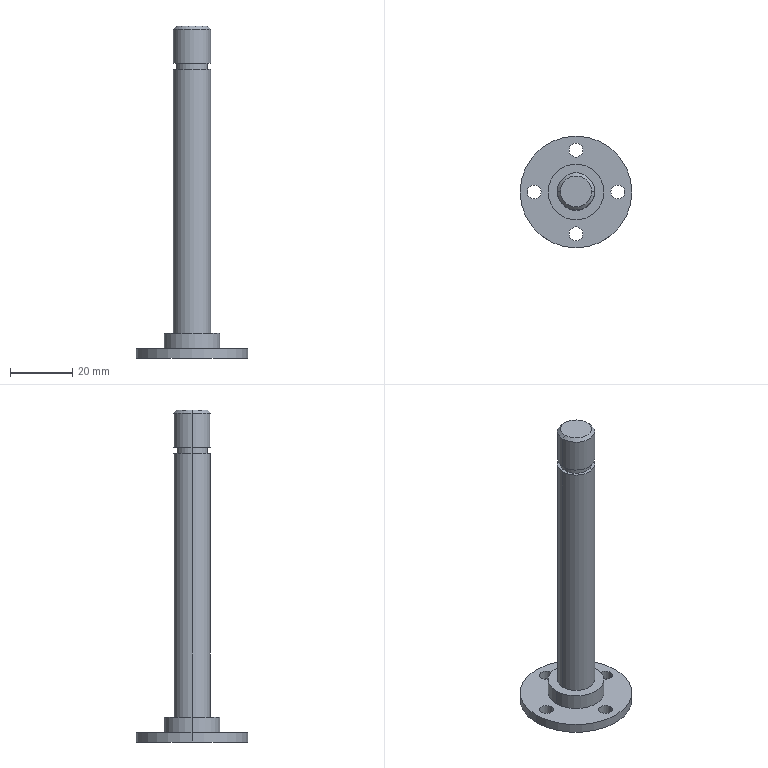Part | STEP file | Floating guide shaft | 1 solid | 26 faces | box 36 x 36 x 107 mm | volume 15245 mm3 | cylinder 18 | plane 6 | cone 2 | commonest cylinder face diameters 4.5 x8 12 x4 10 x2 18 x2 36 x2
STEP:
#1=CARTESIAN_POINT('',(5.,0.,107.));
#2=VERTEX_POINT('',#1);
#3=CARTESIAN_POINT('',(-5.,0.,107.));
#4=VERTEX_POINT('',#3);
#5=CARTESIAN_POINT('',(0.,0.,107.));
#6=DIRECTION('',(0.,0.,1.));
#7=DIRECTION('',(1.,0.,0.));
#8=AXIS2_PLACEMENT_3D('',#5,#6,#7);
#9=CIRCLE('',#8,5.);
#10=EDGE_CURVE('',#2,#4,#9,.T.);
#11=ORIENTED_EDGE('',*,*,#10,.F.);
#12=CARTESIAN_POINT('',(6.,0.,106.));
#13=VERTEX_POINT('',#12);
#14=CARTESIAN_POINT('',(5.,0.,107.));
#15=DIRECTION('',(0.7071,0.,-0.7071));
#16=VECTOR('',#15,1000.);
#17=LINE('',#14,#16);
#18=EDGE_CURVE('',#2,#13,#17,.T.);
#19=ORIENTED_EDGE('',*,*,#18,.T.);
#20=CARTESIAN_POINT('',(-6.,0.,106.));
#21=VERTEX_POINT('',#20);
#22=CARTESIAN_POINT('',(0.,0.,106.));
#23=DIRECTION('',(0.,0.,-1.));
#24=DIRECTION('',(1.,0.,0.));
#25=AXIS2_PLACEMENT_3D('',#22,#23,#24);
#26=CIRCLE('',#25,6.);
#27=EDGE_CURVE('',#21,#13,#26,.T.);
#28=ORIENTED_EDGE('',*,*,#27,.F.);
#29=CARTESIAN_POINT('',(-5.,0.,107.));
#30=DIRECTION('',(-0.7071,0.,-0.7071));
#31=VECTOR('',#30,1000.);
#32=LINE('',#29,#31);
#33=EDGE_CURVE('',#4,#21,#32,.T.);
#34=ORIENTED_EDGE('',*,*,#33,.F.);
#35=EDGE_LOOP('',(#11,#19,#28,#34));
#36=FACE_OUTER_BOUND('',#35,.T.);
#37=CARTESIAN_POINT('',(0.,0.,107.));
#38=DIRECTION('',(0.,0.,-1.));
#39=DIRECTION('',(-1.,0.,0.));
#40=AXIS2_PLACEMENT_3D('',#37,#38,#39);
#41=CONICAL_SURFACE('',#40,5.,0.7854);
#42=ADVANCED_FACE('',(#36),#41,.T.);
#43=ORIENTED_EDGE('',*,*,#27,.T.);
#44=CARTESIAN_POINT('',(6.,0.,95.));
#45=VERTEX_POINT('',#44);
#46=CARTESIAN_POINT('',(6.,0.,107.));
#47=DIRECTION('',(0.,0.,-1.));
#48=VECTOR('',#47,1000.);
#49=LINE('',#46,#48);
#50=EDGE_CURVE('',#13,#45,#49,.T.);
#51=ORIENTED_EDGE('',*,*,#50,.T.);
#52=CARTESIAN_POINT('',(-6.,0.,95.));
#53=VERTEX_POINT('',#52);
#54=CARTESIAN_POINT('',(0.,0.,95.));
#55=DIRECTION('',(0.,0.,1.));
#56=DIRECTION('',(1.,0.,0.));
#57=AXIS2_PLACEMENT_3D('',#54,#55,#56);
#58=CIRCLE('',#57,6.);
#59=EDGE_CURVE('',#45,#53,#58,.T.);
#60=ORIENTED_EDGE('',*,*,#59,.T.);
#61=CARTESIAN_POINT('',(-6.,0.,107.));
#62=DIRECTION('',(0.,0.,-1.));
#63=VECTOR('',#62,1000.);
#64=LINE('',#61,#63);
#65=EDGE_CURVE('',#21,#53,#64,.T.);
#66=ORIENTED_EDGE('',*,*,#65,.F.);
#67=EDGE_LOOP('',(#43,#51,#60,#66));
#68=FACE_OUTER_BOUND('',#67,.T.);
#69=CARTESIAN_POINT('',(0.,0.,107.));
#70=DIRECTION('',(0.,0.,-1.));
#71=DIRECTION('',(-1.,0.,0.));
#72=AXIS2_PLACEMENT_3D('',#69,#70,#71);
#73=CYLINDRICAL_SURFACE('',#72,6.);
#74=ADVANCED_FACE('',(#68),#73,.T.);
#75=CARTESIAN_POINT('',(5.,0.,95.));
#76=VERTEX_POINT('',#75);
#77=CARTESIAN_POINT('',(-5.,0.,95.));
#78=VERTEX_POINT('',#77);
#79=CARTESIAN_POINT('',(0.,0.,95.));
#80=DIRECTION('',(0.,0.,1.));
#81=DIRECTION('',(1.,0.,0.));
#82=AXIS2_PLACEMENT_3D('',#79,#80,#81);
#83=CIRCLE('',#82,5.);
#84=EDGE_CURVE('',#76,#78,#83,.T.);
#85=ORIENTED_EDGE('',*,*,#84,.F.);
#86=CARTESIAN_POINT('',(5.,0.,93.));
#87=VERTEX_POINT('',#86);
#88=CARTESIAN_POINT('',(5.,0.,95.));
#89=DIRECTION('',(0.,0.,-1.));
#90=VECTOR('',#89,1000.);
#91=LINE('',#88,#90);
#92=EDGE_CURVE('',#76,#87,#91,.T.);
#93=ORIENTED_EDGE('',*,*,#92,.T.);
#94=CARTESIAN_POINT('',(-5.,0.,93.));
#95=VERTEX_POINT('',#94);
#96=CARTESIAN_POINT('',(0.,0.,93.));
#97=DIRECTION('',(0.,0.,1.));
#98=DIRECTION('',(1.,0.,0.));
#99=AXIS2_PLACEMENT_3D('',#96,#97,#98);
#100=CIRCLE('',#99,5.);
#101=EDGE_CURVE('',#87,#95,#100,.T.);
#102=ORIENTED_EDGE('',*,*,#101,.T.);
#103=CARTESIAN_POINT('',(-5.,0.,95.));
#104=DIRECTION('',(0.,0.,-1.));
#105=VECTOR('',#104,1000.);
#106=LINE('',#103,#105);
#107=EDGE_CURVE('',#78,#95,#106,.T.);
#108=ORIENTED_EDGE('',*,*,#107,.F.);
#109=EDGE_LOOP('',(#85,#93,#102,#108));
#110=FACE_OUTER_BOUND('',#109,.T.);
#111=CARTESIAN_POINT('',(0.,0.,95.));
#112=DIRECTION('',(0.,0.,-1.));
#113=DIRECTION('',(-1.,0.,0.));
#114=AXIS2_PLACEMENT_3D('',#111,#112,#113);
#115=CYLINDRICAL_SURFACE('',#114,5.);
#116=ADVANCED_FACE('',(#110),#115,.T.);
#117=CARTESIAN_POINT('',(-2.25,13.5,0.));
#118=VERTEX_POINT('',#117);
#119=CARTESIAN_POINT('',(2.25,13.5,0.));
#120=VERTEX_POINT('',#119);
#121=CARTESIAN_POINT('',(0.,13.5,0.));
#122=DIRECTION('',(0.,0.,1.));
#123=DIRECTION('',(1.,0.,0.));
#124=AXIS2_PLACEMENT_3D('',#121,#122,#123);
#125=CIRCLE('',#124,2.25);
#126=EDGE_CURVE('',#118,#120,#125,.T.);
#127=ORIENTED_EDGE('',*,*,#126,.F.);
#128=CARTESIAN_POINT('',(-2.25,13.5,3.));
#129=VERTEX_POINT('',#128);
#130=CARTESIAN_POINT('',(-2.25,13.5,-57.));
#131=DIRECTION('',(0.,0.,1.));
#132=VECTOR('',#131,1000.);
#133=LINE('',#130,#132);
#134=EDGE_CURVE('',#118,#129,#133,.T.);
#135=ORIENTED_EDGE('',*,*,#134,.T.);
#136=CARTESIAN_POINT('',(2.25,13.5,3.));
#137=VERTEX_POINT('',#136);
#138=CARTESIAN_POINT('',(0.,13.5,3.));
#139=DIRECTION('',(0.,0.,1.));
#140=DIRECTION('',(-1.,0.,0.));
#141=AXIS2_PLACEMENT_3D('',#138,#139,#140);
#142=CIRCLE('',#141,2.25);
#143=EDGE_CURVE('',#129,#137,#142,.T.);
#144=ORIENTED_EDGE('',*,*,#143,.T.);
#145=CARTESIAN_POINT('',(2.25,13.5,-57.));
#146=DIRECTION('',(0.,0.,1.));
#147=VECTOR('',#146,1000.);
#148=LINE('',#145,#147);
#149=EDGE_CURVE('',#120,#137,#148,.T.);
#150=ORIENTED_EDGE('',*,*,#149,.F.);
#151=EDGE_LOOP('',(#127,#135,#144,#150));
#152=FACE_OUTER_BOUND('',#151,.T.);
#153=CARTESIAN_POINT('',(0.,13.5,-57.));
#154=DIRECTION('',(0.,0.,1.));
#155=DIRECTION('',(1.,0.,0.));
#156=AXIS2_PLACEMENT_3D('',#153,#154,#155);
#157=CYLINDRICAL_SURFACE('',#156,2.25);
#158=ADVANCED_FACE('',(#152),#157,.F.);
#159=CARTESIAN_POINT('',(-15.75,0.,0.));
#160=VERTEX_POINT('',#159);
#161=CARTESIAN_POINT('',(-11.25,0.,0.));
#162=VERTEX_POINT('',#161);
#163=CARTESIAN_POINT('',(-13.5,0.,0.));
#164=DIRECTION('',(0.,0.,1.));
#165=DIRECTION('',(1.,0.,0.));
#166=AXIS2_PLACEMENT_3D('',#163,#164,#165);
#167=CIRCLE('',#166,2.25);
#168=EDGE_CURVE('',#160,#162,#167,.T.);
#169=ORIENTED_EDGE('',*,*,#168,.F.);
#170=CARTESIAN_POINT('',(-15.75,0.,3.));
#171=VERTEX_POINT('',#170);
#172=CARTESIAN_POINT('',(-15.75,0.,-57.));
#173=DIRECTION('',(0.,0.,1.));
#174=VECTOR('',#173,1000.);
#175=LINE('',#172,#174);
#176=EDGE_CURVE('',#160,#171,#175,.T.);
#177=ORIENTED_EDGE('',*,*,#176,.T.);
#178=CARTESIAN_POINT('',(-11.25,0.,3.));
#179=VERTEX_POINT('',#178);
#180=CARTESIAN_POINT('',(-13.5,0.,3.));
#181=DIRECTION('',(0.,0.,1.));
#182=DIRECTION('',(0.,-1.,0.));
#183=AXIS2_PLACEMENT_3D('',#180,#181,#182);
#184=CIRCLE('',#183,2.25);
#185=EDGE_CURVE('',#171,#179,#184,.T.);
#186=ORIENTED_EDGE('',*,*,#185,.T.);
#187=CARTESIAN_POINT('',(-11.25,0.,-57.));
#188=DIRECTION('',(0.,0.,1.));
#189=VECTOR('',#188,1000.);
#190=LINE('',#187,#189);
#191=EDGE_CURVE('',#162,#179,#190,.T.);
#192=ORIENTED_EDGE('',*,*,#191,.F.);
#193=EDGE_LOOP('',(#169,#177,#186,#192));
#194=FACE_OUTER_BOUND('',#193,.T.);
#195=CARTESIAN_POINT('',(-13.5,0.,-57.));
#196=DIRECTION('',(0.,0.,1.));
#197=DIRECTION('',(1.,0.,0.));
#198=AXIS2_PLACEMENT_3D('',#195,#196,#197);
#199=CYLINDRICAL_SURFACE('',#198,2.25);
#200=ADVANCED_FACE('',(#194),#199,.F.);
#201=CARTESIAN_POINT('',(11.25,0.,0.));
#202=VERTEX_POINT('',#201);
#203=CARTESIAN_POINT('',(15.75,0.,0.));
#204=VERTEX_POINT('',#203);
#205=CARTESIAN_POINT('',(13.5,0.,0.));
#206=DIRECTION('',(0.,0.,1.));
#207=DIRECTION('',(1.,0.,0.));
#208=AXIS2_PLACEMENT_3D('',#205,#206,#207);
#209=CIRCLE('',#208,2.25);
#210=EDGE_CURVE('',#202,#204,#209,.T.);
#211=ORIENTED_EDGE('',*,*,#210,.F.);
#212=CARTESIAN_POINT('',(11.25,0.,3.));
#213=VERTEX_POINT('',#212);
#214=CARTESIAN_POINT('',(11.25,0.,-57.));
#215=DIRECTION('',(0.,0.,1.));
#216=VECTOR('',#215,1000.);
#217=LINE('',#214,#216);
#218=EDGE_CURVE('',#202,#213,#217,.T.);
#219=ORIENTED_EDGE('',*,*,#218,.T.);
#220=CARTESIAN_POINT('',(15.75,0.,3.));
#221=VERTEX_POINT('',#220);
#222=CARTESIAN_POINT('',(13.5,0.,3.));
#223=DIRECTION('',(0.,0.,1.));
#224=DIRECTION('',(0.,1.,0.));
#225=AXIS2_PLACEMENT_3D('',#222,#223,#224);
#226=CIRCLE('',#225,2.25);
#227=EDGE_CURVE('',#213,#221,#226,.T.);
#228=ORIENTED_EDGE('',*,*,#227,.T.);
#229=CARTESIAN_POINT('',(15.75,0.,-57.));
#230=DIRECTION('',(0.,0.,1.));
#231=VECTOR('',#230,1000.);
#232=LINE('',#229,#231);
#233=EDGE_CURVE('',#204,#221,#232,.T.);
#234=ORIENTED_EDGE('',*,*,#233,.F.);
#235=EDGE_LOOP('',(#211,#219,#228,#234));
#236=FACE_OUTER_BOUND('',#235,.T.);
#237=CARTESIAN_POINT('',(13.5,0.,-57.));
#238=DIRECTION('',(0.,0.,1.));
#239=DIRECTION('',(1.,0.,0.));
#240=AXIS2_PLACEMENT_3D('',#237,#238,#239);
#241=CYLINDRICAL_SURFACE('',#240,2.25);
#242=ADVANCED_FACE('',(#236),#241,.F.);
#243=CARTESIAN_POINT('',(6.,0.,93.));
#244=VERTEX_POINT('',#243);
#245=CARTESIAN_POINT('',(-6.,0.,93.));
#246=VERTEX_POINT('',#245);
#247=CARTESIAN_POINT('',(0.,0.,93.));
#248=DIRECTION('',(0.,0.,1.));
#249=DIRECTION('',(1.,0.,0.));
#250=AXIS2_PLACEMENT_3D('',#247,#248,#249);
#251=CIRCLE('',#250,6.);
#252=EDGE_CURVE('',#244,#246,#251,.T.);
#253=ORIENTED_EDGE('',*,*,#252,.F.);
#254=CARTESIAN_POINT('',(6.,0.,8.));
#255=VERTEX_POINT('',#254);
#256=CARTESIAN_POINT('',(6.,0.,93.));
#257=DIRECTION('',(0.,0.,-1.));
#258=VECTOR('',#257,1000.);
#259=LINE('',#256,#258);
#260=EDGE_CURVE('',#244,#255,#259,.T.);
#261=ORIENTED_EDGE('',*,*,#260,.T.);
#262=CARTESIAN_POINT('',(-6.,0.,8.));
#263=VERTEX_POINT('',#262);
#264=CARTESIAN_POINT('',(0.,0.,8.));
#265=DIRECTION('',(0.,0.,1.));
#266=DIRECTION('',(1.,0.,0.));
#267=AXIS2_PLACEMENT_3D('',#264,#265,#266);
#268=CIRCLE('',#267,6.);
#269=EDGE_CURVE('',#255,#263,#268,.T.);
#270=ORIENTED_EDGE('',*,*,#269,.T.);
#271=CARTESIAN_POINT('',(-6.,0.,93.));
#272=DIRECTION('',(0.,0.,-1.));
#273=VECTOR('',#272,1000.);
#274=LINE('',#271,#273);
#275=EDGE_CURVE('',#246,#263,#274,.T.);
#276=ORIENTED_EDGE('',*,*,#275,.F.);
#277=EDGE_LOOP('',(#253,#261,#270,#276));
#278=FACE_OUTER_BOUND('',#277,.T.);
#279=CARTESIAN_POINT('',(0.,0.,93.));
#280=DIRECTION('',(0.,0.,-1.));
#281=DIRECTION('',(-1.,0.,0.));
#282=AXIS2_PLACEMENT_3D('',#279,#280,#281);
#283=CYLINDRICAL_SURFACE('',#282,6.);
#284=ADVANCED_FACE('',(#278),#283,.T.);
#285=CARTESIAN_POINT('',(-2.25,-13.5,0.));
#286=VERTEX_POINT('',#285);
#287=CARTESIAN_POINT('',(2.25,-13.5,0.));
#288=VERTEX_POINT('',#287);
#289=CARTESIAN_POINT('',(0.,-13.5,0.));
#290=DIRECTION('',(0.,0.,1.));
#291=DIRECTION('',(1.,0.,0.));
#292=AXIS2_PLACEMENT_3D('',#289,#290,#291);
#293=CIRCLE('',#292,2.25);
#294=EDGE_CURVE('',#286,#288,#293,.T.);
#295=ORIENTED_EDGE('',*,*,#294,.F.);
#296=CARTESIAN_POINT('',(-2.25,-13.5,3.));
#297=VERTEX_POINT('',#296);
#298=CARTESIAN_POINT('',(-2.25,-13.5,-57.));
#299=DIRECTION('',(0.,0.,1.));
#300=VECTOR('',#299,1000.);
#301=LINE('',#298,#300);
#302=EDGE_CURVE('',#286,#297,#301,.T.);
#303=ORIENTED_EDGE('',*,*,#302,.T.);
#304=CARTESIAN_POINT('',(2.25,-13.5,3.));
#305=VERTEX_POINT('',#304);
#306=CARTESIAN_POINT('',(0.,-13.5,3.));
#307=DIRECTION('',(0.,0.,1.));
#308=DIRECTION('',(1.,0.,0.));
#309=AXIS2_PLACEMENT_3D('',#306,#307,#308);
#310=CIRCLE('',#309,2.25);
#311=EDGE_CURVE('',#297,#305,#310,.T.);
#312=ORIENTED_EDGE('',*,*,#311,.T.);
#313=CARTESIAN_POINT('',(2.25,-13.5,-57.));
#314=DIRECTION('',(0.,0.,1.));
#315=VECTOR('',#314,1000.);
#316=LINE('',#313,#315);
#317=EDGE_CURVE('',#288,#305,#316,.T.);
#318=ORIENTED_EDGE('',*,*,#317,.F.);
#319=EDGE_LOOP('',(#295,#303,#312,#318));
#320=FACE_OUTER_BOUND('',#319,.T.);
#321=CARTESIAN_POINT('',(0.,-13.5,-57.));
#322=DIRECTION('',(0.,0.,1.));
#323=DIRECTION('',(1.,0.,0.));
#324=AXIS2_PLACEMENT_3D('',#321,#322,#323);
#325=CYLINDRICAL_SURFACE('',#324,2.25);
#326=ADVANCED_FACE('',(#320),#325,.F.);
#327=CARTESIAN_POINT('',(9.,0.,8.));
#328=VERTEX_POINT('',#327);
#329=CARTESIAN_POINT('',(-9.,0.,8.));
#330=VERTEX_POINT('',#329);
#331=CARTESIAN_POINT('',(0.,0.,8.));
#332=DIRECTION('',(0.,0.,1.));
#333=DIRECTION('',(1.,0.,0.));
#334=AXIS2_PLACEMENT_3D('',#331,#332,#333);
#335=CIRCLE('',#334,9.);
#336=EDGE_CURVE('',#328,#330,#335,.T.);
#337=ORIENTED_EDGE('',*,*,#336,.F.);
#338=CARTESIAN_POINT('',(9.,0.,3.));
#339=VERTEX_POINT('',#338);
#340=CARTESIAN_POINT('',(9.,0.,8.));
#341=DIRECTION('',(0.,0.,-1.));
#342=VECTOR('',#341,1000.);
#343=LINE('',#340,#342);
#344=EDGE_CURVE('',#328,#339,#343,.T.);
#345=ORIENTED_EDGE('',*,*,#344,.T.);
#346=CARTESIAN_POINT('',(-9.,0.,3.));
#347=VERTEX_POINT('',#346);
#348=CARTESIAN_POINT('',(0.,0.,3.));
#349=DIRECTION('',(0.,0.,1.));
#350=DIRECTION('',(1.,0.,0.));
#351=AXIS2_PLACEMENT_3D('',#348,#349,#350);
#352=CIRCLE('',#351,9.);
#353=EDGE_CURVE('',#339,#347,#352,.T.);
#354=ORIENTED_EDGE('',*,*,#353,.T.);
#355=CARTESIAN_POINT('',(-9.,0.,8.));
#356=DIRECTION('',(0.,0.,-1.));
#357=VECTOR('',#356,1000.);
#358=LINE('',#355,#357);
#359=EDGE_CURVE('',#330,#347,#358,.T.);
#360=ORIENTED_EDGE('',*,*,#359,.F.);
#361=EDGE_LOOP('',(#337,#345,#354,#360));
#362=FACE_OUTER_BOUND('',#361,.T.);
#363=CARTESIAN_POINT('',(0.,0.,8.));
#364=DIRECTION('',(0.,0.,-1.));
#365=DIRECTION('',(-1.,0.,0.));
#366=AXIS2_PLACEMENT_3D('',#363,#364,#365);
#367=CYLINDRICAL_SURFACE('',#366,9.);
#368=ADVANCED_FACE('',(#362),#367,.T.);
#369=CARTESIAN_POINT('',(18.,0.,3.));
#370=VERTEX_POINT('',#369);
#371=CARTESIAN_POINT('',(-18.,0.,3.));
#372=VERTEX_POINT('',#371);
#373=CARTESIAN_POINT('',(0.,0.,3.));
#374=DIRECTION('',(0.,0.,1.));
#375=DIRECTION('',(1.,0.,0.));
#376=AXIS2_PLACEMENT_3D('',#373,#374,#375);
#377=CIRCLE('',#376,18.);
#378=EDGE_CURVE('',#370,#372,#377,.T.);
#379=ORIENTED_EDGE('',*,*,#378,.F.);
#380=CARTESIAN_POINT('',(18.,0.,0.));
#381=VERTEX_POINT('',#380);
#382=CARTESIAN_POINT('',(18.,0.,3.));
#383=DIRECTION('',(0.,0.,-1.));
#384=VECTOR('',#383,1000.);
#385=LINE('',#382,#384);
#386=EDGE_CURVE('',#370,#381,#385,.T.);
#387=ORIENTED_EDGE('',*,*,#386,.T.);
#388=CARTESIAN_POINT('',(-18.,0.,0.));
#389=VERTEX_POINT('',#388);
#390=CARTESIAN_POINT('',(0.,0.,0.));
#391=DIRECTION('',(0.,0.,1.));
#392=DIRECTION('',(1.,0.,0.));
#393=AXIS2_PLACEMENT_3D('',#390,#391,#392);
#394=CIRCLE('',#393,18.);
#395=EDGE_CURVE('',#381,#389,#394,.T.);
#396=ORIENTED_EDGE('',*,*,#395,.T.);
#397=CARTESIAN_POINT('',(-18.,0.,3.));
#398=DIRECTION('',(0.,0.,-1.));
#399=VECTOR('',#398,1000.);
#400=LINE('',#397,#399);
#401=EDGE_CURVE('',#372,#389,#400,.T.);
#402=ORIENTED_EDGE('',*,*,#401,.F.);
#403=EDGE_LOOP('',(#379,#387,#396,#402));
#404=FACE_OUTER_BOUND('',#403,.T.);
#405=CARTESIAN_POINT('',(0.,0.,3.));
#406=DIRECTION('',(0.,0.,-1.));
#407=DIRECTION('',(-1.,0.,0.));
#408=AXIS2_PLACEMENT_3D('',#405,#406,#407);
#409=CYLINDRICAL_SURFACE('',#408,18.);
#410=ADVANCED_FACE('',(#404),#409,.T.);
#411=ORIENTED_EDGE('',*,*,#386,.F.);
#412=CARTESIAN_POINT('',(0.,0.,3.));
#413=DIRECTION('',(0.,0.,1.));
#414=DIRECTION('',(1.,0.,0.));
#415=AXIS2_PLACEMENT_3D('',#412,#413,#414);
#416=CIRCLE('',#415,18.);
#417=EDGE_CURVE('',#372,#370,#416,.T.);
#418=ORIENTED_EDGE('',*,*,#417,.F.);
#419=ORIENTED_EDGE('',*,*,#401,.T.);
#420=CARTESIAN_POINT('',(0.,0.,0.));
#421=DIRECTION('',(0.,0.,1.));
#422=DIRECTION('',(1.,0.,0.));
#423=AXIS2_PLACEMENT_3D('',#420,#421,#422);
#424=CIRCLE('',#423,18.);
#425=EDGE_CURVE('',#389,#381,#424,.T.);
#426=ORIENTED_EDGE('',*,*,#425,.T.);
#427=EDGE_LOOP('',(#411,#418,#419,#426));
#428=FACE_OUTER_BOUND('',#427,.T.);
#429=CARTESIAN_POINT('',(0.,0.,3.));
#430=DIRECTION('',(0.,0.,-1.));
#431=DIRECTION('',(-1.,0.,0.));
#432=AXIS2_PLACEMENT_3D('',#429,#430,#431);
#433=CYLINDRICAL_SURFACE('',#432,18.);
#434=ADVANCED_FACE('',(#428),#433,.T.);
#435=CARTESIAN_POINT('',(0.,13.5,3.));
#436=DIRECTION('',(0.,0.,1.));
#437=DIRECTION('',(-1.,0.,0.));
#438=AXIS2_PLACEMENT_3D('',#435,#436,#437);
#439=CIRCLE('',#438,2.25);
#440=EDGE_CURVE('',#137,#129,#439,.T.);
#441=ORIENTED_EDGE('',*,*,#440,.F.);
#442=ORIENTED_EDGE('',*,*,#143,.F.);
#443=EDGE_LOOP('',(#441,#442));
#444=FACE_BOUND('',#443,.T.);
#445=CARTESIAN_POINT('',(-13.5,0.,3.));
#446=DIRECTION('',(0.,0.,1.));
#447=DIRECTION('',(0.,-1.,0.));
#448=AXIS2_PLACEMENT_3D('',#445,#446,#447);
#449=CIRCLE('',#448,2.25);
#450=EDGE_CURVE('',#179,#171,#449,.T.);
#451=ORIENTED_EDGE('',*,*,#450,.F.);
#452=ORIENTED_EDGE('',*,*,#185,.F.);
#453=EDGE_LOOP('',(#451,#452));
#454=FACE_BOUND('',#453,.T.);
#455=CARTESIAN_POINT('',(13.5,0.,3.));
#456=DIRECTION('',(0.,0.,1.));
#457=DIRECTION('',(0.,1.,0.));
#458=AXIS2_PLACEMENT_3D('',#455,#456,#457);
#459=CIRCLE('',#458,2.25);
#460=EDGE_CURVE('',#221,#213,#459,.T.);
#461=ORIENTED_EDGE('',*,*,#460,.F.);
#462=ORIENTED_EDGE('',*,*,#227,.F.);
#463=EDGE_LOOP('',(#461,#462));
#464=FACE_BOUND('',#463,.T.);
#465=CARTESIAN_POINT('',(0.,-13.5,3.));
#466=DIRECTION('',(0.,0.,1.));
#467=DIRECTION('',(1.,0.,0.));
#468=AXIS2_PLACEMENT_3D('',#465,#466,#467);
#469=CIRCLE('',#468,2.25);
#470=EDGE_CURVE('',#305,#297,#469,.T.);
#471=ORIENTED_EDGE('',*,*,#470,.F.);
#472=ORIENTED_EDGE('',*,*,#311,.F.);
#473=EDGE_LOOP('',(#471,#472));
#474=FACE_BOUND('',#473,.T.);
#475=CARTESIAN_POINT('',(0.,0.,3.));
#476=DIRECTION('',(0.,0.,1.));
#477=DIRECTION('',(1.,0.,0.));
#478=AXIS2_PLACEMENT_3D('',#475,#476,#477);
#479=CIRCLE('',#478,9.);
#480=EDGE_CURVE('',#347,#339,#479,.T.);
#481=ORIENTED_EDGE('',*,*,#480,.F.);
#482=ORIENTED_EDGE('',*,*,#353,.F.);
#483=EDGE_LOOP('',(#481,#482));
#484=FACE_BOUND('',#483,.T.);
#485=ORIENTED_EDGE('',*,*,#417,.T.);
#486=ORIENTED_EDGE('',*,*,#378,.T.);
#487=EDGE_LOOP('',(#485,#486));
#488=FACE_OUTER_BOUND('',#487,.T.);
#489=CARTESIAN_POINT('',(0.,0.,3.));
#490=DIRECTION('',(0.,0.,1.));
#491=DIRECTION('',(1.,0.,0.));
#492=AXIS2_PLACEMENT_3D('',#489,#490,#491);
#493=PLANE('',#492);
#494=ADVANCED_FACE('',(#444,#454,#464,#474,#484,#488),#493,.T.);
#495=CARTESIAN_POINT('',(0.,13.5,0.));
#496=DIRECTION('',(0.,0.,1.));
#497=DIRECTION('',(1.,0.,0.));
#498=AXIS2_PLACEMENT_3D('',#495,#496,#497);
#499=CIRCLE('',#498,2.25);
#500=EDGE_CURVE('',#120,#118,#499,.T.);
#501=ORIENTED_EDGE('',*,*,#500,.T.);
#502=ORIENTED_EDGE('',*,*,#126,.T.);
#503=EDGE_LOOP('',(#501,#502));
#504=FACE_BOUND('',#503,.T.);
#505=CARTESIAN_POINT('',(-13.5,0.,0.));
#506=DIRECTION('',(0.,0.,1.));
#507=DIRECTION('',(1.,0.,0.));
#508=AXIS2_PLACEMENT_3D('',#505,#506,#507);
#509=CIRCLE('',#508,2.25);
#510=EDGE_CURVE('',#162,#160,#509,.T.);
#511=ORIENTED_EDGE('',*,*,#510,.T.);
#512=ORIENTED_EDGE('',*,*,#168,.T.);
#513=EDGE_LOOP('',(#511,#512));
#514=FACE_BOUND('',#513,.T.);
#515=CARTESIAN_POINT('',(13.5,0.,0.));
#516=DIRECTION('',(0.,0.,1.));
#517=DIRECTION('',(1.,0.,0.));
#518=AXIS2_PLACEMENT_3D('',#515,#516,#517);
#519=CIRCLE('',#518,2.25);
#520=EDGE_CURVE('',#204,#202,#519,.T.);
#521=ORIENTED_EDGE('',*,*,#520,.T.);
#522=ORIENTED_EDGE('',*,*,#210,.T.);
#523=EDGE_LOOP('',(#521,#522));
#524=FACE_BOUND('',#523,.T.);
#525=CARTESIAN_POINT('',(0.,-13.5,0.));
#526=DIRECTION('',(0.,0.,1.));
#527=DIRECTION('',(1.,0.,0.));
#528=AXIS2_PLACEMENT_3D('',#525,#526,#527);
#529=CIRCLE('',#528,2.25);
#530=EDGE_CURVE('',#288,#286,#529,.T.);
#531=ORIENTED_EDGE('',*,*,#530,.T.);
#532=ORIENTED_EDGE('',*,*,#294,.T.);
#533=EDGE_LOOP('',(#531,#532));
#534=FACE_BOUND('',#533,.T.);
#535=ORIENTED_EDGE('',*,*,#425,.F.);
#536=ORIENTED_EDGE('',*,*,#395,.F.);
#537=EDGE_LOOP('',(#535,#536));
#538=FACE_OUTER_BOUND('',#537,.T.);
#539=CARTESIAN_POINT('',(0.,0.,0.));
#540=DIRECTION('',(0.,0.,1.));
#541=DIRECTION('',(1.,0.,0.));
#542=AXIS2_PLACEMENT_3D('',#539,#540,#541);
#543=PLANE('',#542);
#544=ADVANCED_FACE('',(#504,#514,#524,#534,#538),#543,.F.);
#545=ORIENTED_EDGE('',*,*,#344,.F.);
#546=CARTESIAN_POINT('',(0.,0.,8.));
#547=DIRECTION('',(0.,0.,1.));
#548=DIRECTION('',(1.,0.,0.));
#549=AXIS2_PLACEMENT_3D('',#546,#547,#548);
#550=CIRCLE('',#549,9.);
#551=EDGE_CURVE('',#330,#328,#550,.T.);
#552=ORIENTED_EDGE('',*,*,#551,.F.);
#553=ORIENTED_EDGE('',*,*,#359,.T.);
#554=ORIENTED_EDGE('',*,*,#480,.T.);
#555=EDGE_LOOP('',(#545,#552,#553,#554));
#556=FACE_OUTER_BOUND('',#555,.T.);
#557=CARTESIAN_POINT('',(0.,0.,8.));
#558=DIRECTION('',(0.,0.,-1.));
#559=DIRECTION('',(-1.,0.,0.));
#560=AXIS2_PLACEMENT_3D('',#557,#558,#559);
#561=CYLINDRICAL_SURFACE('',#560,9.);
#562=ADVANCED_FACE('',(#556),#561,.T.);
#563=CARTESIAN_POINT('',(0.,0.,8.));
#564=DIRECTION('',(0.,0.,1.));
#565=DIRECTION('',(1.,0.,0.));
#566=AXIS2_PLACEMENT_3D('',#563,#564,#565);
#567=CIRCLE('',#566,6.);
#568=EDGE_CURVE('',#263,#255,#567,.T.);
#569=ORIENTED_EDGE('',*,*,#568,.F.);
#570=ORIENTED_EDGE('',*,*,#269,.F.);
#571=EDGE_LOOP('',(#569,#570));
#572=FACE_BOUND('',#571,.T.);
#573=ORIENTED_EDGE('',*,*,#551,.T.);
#574=ORIENTED_EDGE('',*,*,#336,.T.);
#575=EDGE_LOOP('',(#573,#574));
#576=FACE_OUTER_BOUND('',#575,.T.);
#577=CARTESIAN_POINT('',(0.,0.,8.));
#578=DIRECTION('',(0.,0.,1.));
#579=DIRECTION('',(1.,0.,0.));
#580=AXIS2_PLACEMENT_3D('',#577,#578,#579);
#581=PLANE('',#580);
#582=ADVANCED_FACE('',(#572,#576),#581,.T.);
#583=ORIENTED_EDGE('',*,*,#302,.F.);
#584=ORIENTED_EDGE('',*,*,#530,.F.);
#585=ORIENTED_EDGE('',*,*,#317,.T.);
#586=ORIENTED_EDGE('',*,*,#470,.T.);
#587=EDGE_LOOP('',(#583,#584,#585,#586));
#588=FACE_OUTER_BOUND('',#587,.T.);
#589=CARTESIAN_POINT('',(0.,-13.5,-57.));
#590=DIRECTION('',(0.,0.,1.));
#591=DIRECTION('',(1.,0.,0.));
#592=AXIS2_PLACEMENT_3D('',#589,#590,#591);
#593=CYLINDRICAL_SURFACE('',#592,2.25);
#594=ADVANCED_FACE('',(#588),#593,.F.);
#595=ORIENTED_EDGE('',*,*,#260,.F.);
#596=CARTESIAN_POINT('',(0.,0.,93.));
#597=DIRECTION('',(0.,0.,1.));
#598=DIRECTION('',(1.,0.,0.));
#599=AXIS2_PLACEMENT_3D('',#596,#597,#598);
#600=CIRCLE('',#599,6.);
#601=EDGE_CURVE('',#246,#244,#600,.T.);
#602=ORIENTED_EDGE('',*,*,#601,.F.);
#603=ORIENTED_EDGE('',*,*,#275,.T.);
#604=ORIENTED_EDGE('',*,*,#568,.T.);
#605=EDGE_LOOP('',(#595,#602,#603,#604));
#606=FACE_OUTER_BOUND('',#605,.T.);
#607=CARTESIAN_POINT('',(0.,0.,93.));
#608=DIRECTION('',(0.,0.,-1.));
#609=DIRECTION('',(-1.,0.,0.));
#610=AXIS2_PLACEMENT_3D('',#607,#608,#609);
#611=CYLINDRICAL_SURFACE('',#610,6.);
#612=ADVANCED_FACE('',(#606),#611,.T.);
#613=CARTESIAN_POINT('',(0.,0.,93.));
#614=DIRECTION('',(0.,0.,1.));
#615=DIRECTION('',(1.,0.,0.));
#616=AXIS2_PLACEMENT_3D('',#613,#614,#615);
#617=CIRCLE('',#616,5.);
#618=EDGE_CURVE('',#95,#87,#617,.T.);
#619=ORIENTED_EDGE('',*,*,#618,.F.);
#620=ORIENTED_EDGE('',*,*,#101,.F.);
#621=EDGE_LOOP('',(#619,#620));
#622=FACE_BOUND('',#621,.T.);
#623=ORIENTED_EDGE('',*,*,#601,.T.);
#624=ORIENTED_EDGE('',*,*,#252,.T.);
#625=EDGE_LOOP('',(#623,#624));
#626=FACE_OUTER_BOUND('',#625,.T.);
#627=CARTESIAN_POINT('',(0.,0.,93.));
#628=DIRECTION('',(0.,0.,1.));
#629=DIRECTION('',(1.,0.,0.));
#630=AXIS2_PLACEMENT_3D('',#627,#628,#629);
#631=PLANE('',#630);
#632=ADVANCED_FACE('',(#622,#626),#631,.T.);
#633=ORIENTED_EDGE('',*,*,#218,.F.);
#634=ORIENTED_EDGE('',*,*,#520,.F.);
#635=ORIENTED_EDGE('',*,*,#233,.T.);
#636=ORIENTED_EDGE('',*,*,#460,.T.);
#637=EDGE_LOOP('',(#633,#634,#635,#636));
#638=FACE_OUTER_BOUND('',#637,.T.);
#639=CARTESIAN_POINT('',(13.5,0.,-57.));
#640=DIRECTION('',(0.,0.,1.));
#641=DIRECTION('',(1.,0.,0.));
#642=AXIS2_PLACEMENT_3D('',#639,#640,#641);
#643=CYLINDRICAL_SURFACE('',#642,2.25);
#644=ADVANCED_FACE('',(#638),#643,.F.);
#645=ORIENTED_EDGE('',*,*,#176,.F.);
#646=ORIENTED_EDGE('',*,*,#510,.F.);
#647=ORIENTED_EDGE('',*,*,#191,.T.);
#648=ORIENTED_EDGE('',*,*,#450,.T.);
#649=EDGE_LOOP('',(#645,#646,#647,#648));
#650=FACE_OUTER_BOUND('',#649,.T.);
#651=CARTESIAN_POINT('',(-13.5,0.,-57.));
#652=DIRECTION('',(0.,0.,1.));
#653=DIRECTION('',(1.,0.,0.));
#654=AXIS2_PLACEMENT_3D('',#651,#652,#653);
#655=CYLINDRICAL_SURFACE('',#654,2.25);
#656=ADVANCED_FACE('',(#650),#655,.F.);
#657=ORIENTED_EDGE('',*,*,#134,.F.);
#658=ORIENTED_EDGE('',*,*,#500,.F.);
#659=ORIENTED_EDGE('',*,*,#149,.T.);
#660=ORIENTED_EDGE('',*,*,#440,.T.);
#661=EDGE_LOOP('',(#657,#658,#659,#660));
#662=FACE_OUTER_BOUND('',#661,.T.);
#663=CARTESIAN_POINT('',(0.,13.5,-57.));
#664=DIRECTION('',(0.,0.,1.));
#665=DIRECTION('',(1.,0.,0.));
#666=AXIS2_PLACEMENT_3D('',#663,#664,#665);
#667=CYLINDRICAL_SURFACE('',#666,2.25);
#668=ADVANCED_FACE('',(#662),#667,.F.);
#669=ORIENTED_EDGE('',*,*,#92,.F.);
#670=CARTESIAN_POINT('',(0.,0.,95.));
#671=DIRECTION('',(0.,0.,1.));
#672=DIRECTION('',(1.,0.,0.));
#673=AXIS2_PLACEMENT_3D('',#670,#671,#672);
#674=CIRCLE('',#673,5.);
#675=EDGE_CURVE('',#78,#76,#674,.T.);
#676=ORIENTED_EDGE('',*,*,#675,.F.);
#677=ORIENTED_EDGE('',*,*,#107,.T.);
#678=ORIENTED_EDGE('',*,*,#618,.T.);
#679=EDGE_LOOP('',(#669,#676,#677,#678));
#680=FACE_OUTER_BOUND('',#679,.T.);
#681=CARTESIAN_POINT('',(0.,0.,95.));
#682=DIRECTION('',(0.,0.,-1.));
#683=DIRECTION('',(-1.,0.,0.));
#684=AXIS2_PLACEMENT_3D('',#681,#682,#683);
#685=CYLINDRICAL_SURFACE('',#684,5.);
#686=ADVANCED_FACE('',(#680),#685,.T.);
#687=ORIENTED_EDGE('',*,*,#50,.F.);
#688=CARTESIAN_POINT('',(0.,0.,106.));
#689=DIRECTION('',(0.,0.,-1.));
#690=DIRECTION('',(1.,0.,0.));
#691=AXIS2_PLACEMENT_3D('',#688,#689,#690);
#692=CIRCLE('',#691,6.);
#693=EDGE_CURVE('',#13,#21,#692,.T.);
#694=ORIENTED_EDGE('',*,*,#693,.T.);
#695=ORIENTED_EDGE('',*,*,#65,.T.);
#696=CARTESIAN_POINT('',(0.,0.,95.));
#697=DIRECTION('',(0.,0.,1.));
#698=DIRECTION('',(1.,0.,0.));
#699=AXIS2_PLACEMENT_3D('',#696,#697,#698);
#700=CIRCLE('',#699,6.);
#701=EDGE_CURVE('',#53,#45,#700,.T.);
#702=ORIENTED_EDGE('',*,*,#701,.T.);
#703=EDGE_LOOP('',(#687,#694,#695,#702));
#704=FACE_OUTER_BOUND('',#703,.T.);
#705=CARTESIAN_POINT('',(0.,0.,107.));
#706=DIRECTION('',(0.,0.,-1.));
#707=DIRECTION('',(-1.,0.,0.));
#708=AXIS2_PLACEMENT_3D('',#705,#706,#707);
#709=CYLINDRICAL_SURFACE('',#708,6.);
#710=ADVANCED_FACE('',(#704),#709,.T.);
#711=CARTESIAN_POINT('',(0.,0.,107.));
#712=DIRECTION('',(0.,0.,1.));
#713=DIRECTION('',(1.,0.,0.));
#714=AXIS2_PLACEMENT_3D('',#711,#712,#713);
#715=CIRCLE('',#714,5.);
#716=EDGE_CURVE('',#4,#2,#715,.T.);
#717=ORIENTED_EDGE('',*,*,#716,.T.);
#718=ORIENTED_EDGE('',*,*,#10,.T.);
#719=EDGE_LOOP('',(#717,#718));
#720=FACE_OUTER_BOUND('',#719,.T.);
#721=CARTESIAN_POINT('',(0.,0.,107.));
#722=DIRECTION('',(0.,0.,1.));
#723=DIRECTION('',(1.,0.,0.));
#724=AXIS2_PLACEMENT_3D('',#721,#722,#723);
#725=PLANE('',#724);
#726=ADVANCED_FACE('',(#720),#725,.T.);
#727=ORIENTED_EDGE('',*,*,#675,.T.);
#728=ORIENTED_EDGE('',*,*,#84,.T.);
#729=EDGE_LOOP('',(#727,#728));
#730=FACE_BOUND('',#729,.T.);
#731=ORIENTED_EDGE('',*,*,#701,.F.);
#732=ORIENTED_EDGE('',*,*,#59,.F.);
#733=EDGE_LOOP('',(#731,#732));
#734=FACE_OUTER_BOUND('',#733,.T.);
#735=CARTESIAN_POINT('',(0.,0.,95.));
#736=DIRECTION('',(0.,0.,1.));
#737=DIRECTION('',(1.,0.,0.));
#738=AXIS2_PLACEMENT_3D('',#735,#736,#737);
#739=PLANE('',#738);
#740=ADVANCED_FACE('',(#730,#734),#739,.F.);
#741=ORIENTED_EDGE('',*,*,#18,.F.);
#742=ORIENTED_EDGE('',*,*,#716,.F.);
#743=ORIENTED_EDGE('',*,*,#33,.T.);
#744=ORIENTED_EDGE('',*,*,#693,.F.);
#745=EDGE_LOOP('',(#741,#742,#743,#744));
#746=FACE_OUTER_BOUND('',#745,.T.);
#747=CARTESIAN_POINT('',(0.,0.,107.));
#748=DIRECTION('',(0.,0.,-1.));
#749=DIRECTION('',(-1.,0.,0.));
#750=AXIS2_PLACEMENT_3D('',#747,#748,#749);
#751=CONICAL_SURFACE('',#750,5.,0.7854);
#752=ADVANCED_FACE('',(#746),#751,.T.);
#753=CLOSED_SHELL('',(#42,#74,#116,#158,#200,#242,#284,#326,#368,#410,#434,#494,#544,#562,#582,#594,#612,#632,#644,#656,#668,#686,#710,#726,#740,#752));
#754=MANIFOLD_SOLID_BREP('',#753);
#755=CARTESIAN_POINT('',(0.,0.,0.));
#756=DIRECTION('',(0.,0.,1.));
#757=DIRECTION('',(1.,0.,0.));
#758=AXIS2_PLACEMENT_3D('',#755,#756,#757);
#759=(LENGTH_UNIT()NAMED_UNIT(*)SI_UNIT(.MILLI.,.METRE.));
#760=UNCERTAINTY_MEASURE_WITH_UNIT(LENGTH_MEASURE(0.00001),#759,'','');
#761=(NAMED_UNIT(*)PLANE_ANGLE_UNIT()SI_UNIT($,.RADIAN.));
#762=(NAMED_UNIT(*)SI_UNIT($,.STERADIAN.)SOLID_ANGLE_UNIT());
#763=(GEOMETRIC_REPRESENTATION_CONTEXT(3)GLOBAL_UNCERTAINTY_ASSIGNED_CONTEXT((#760))GLOBAL_UNIT_ASSIGNED_CONTEXT((#759,#761,#762))REPRESENTATION_CONTEXT('',''));
#764=ADVANCED_BREP_SHAPE_REPRESENTATION('',(#754,#758),#763);